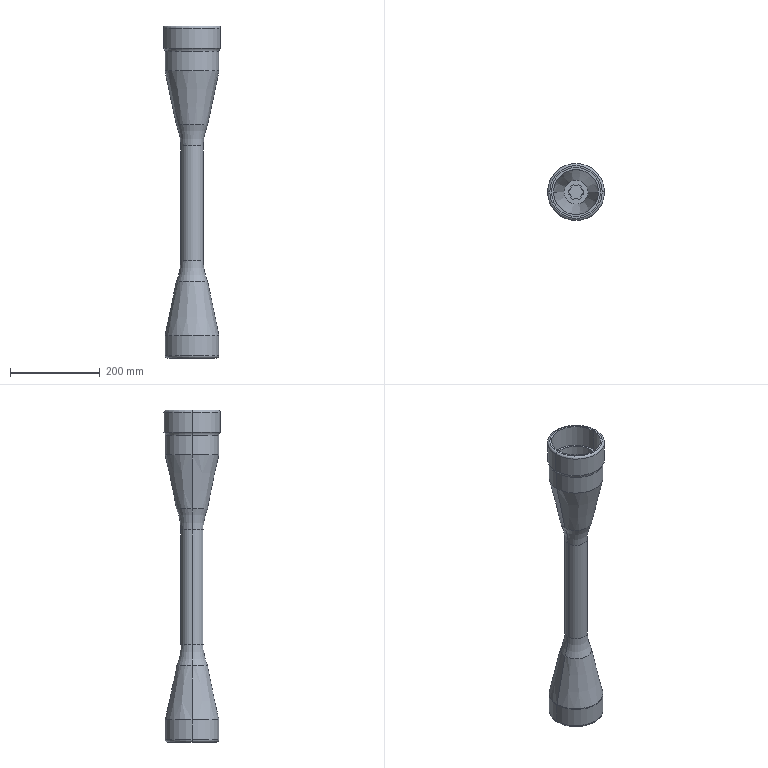Part | STEP file | SHAFT_DIA30_CARDAN2V11 | 2 solids | 121 faces | box 126.77 x 126.77 x 738.528 mm | volume 1857517 mm3 | plane 57 | cylinder 44 | torus 12 | cone 8 | commonest cylinder face diameters 34 x14 28 x12 100 x4 120 x4 30 x2 40 x2